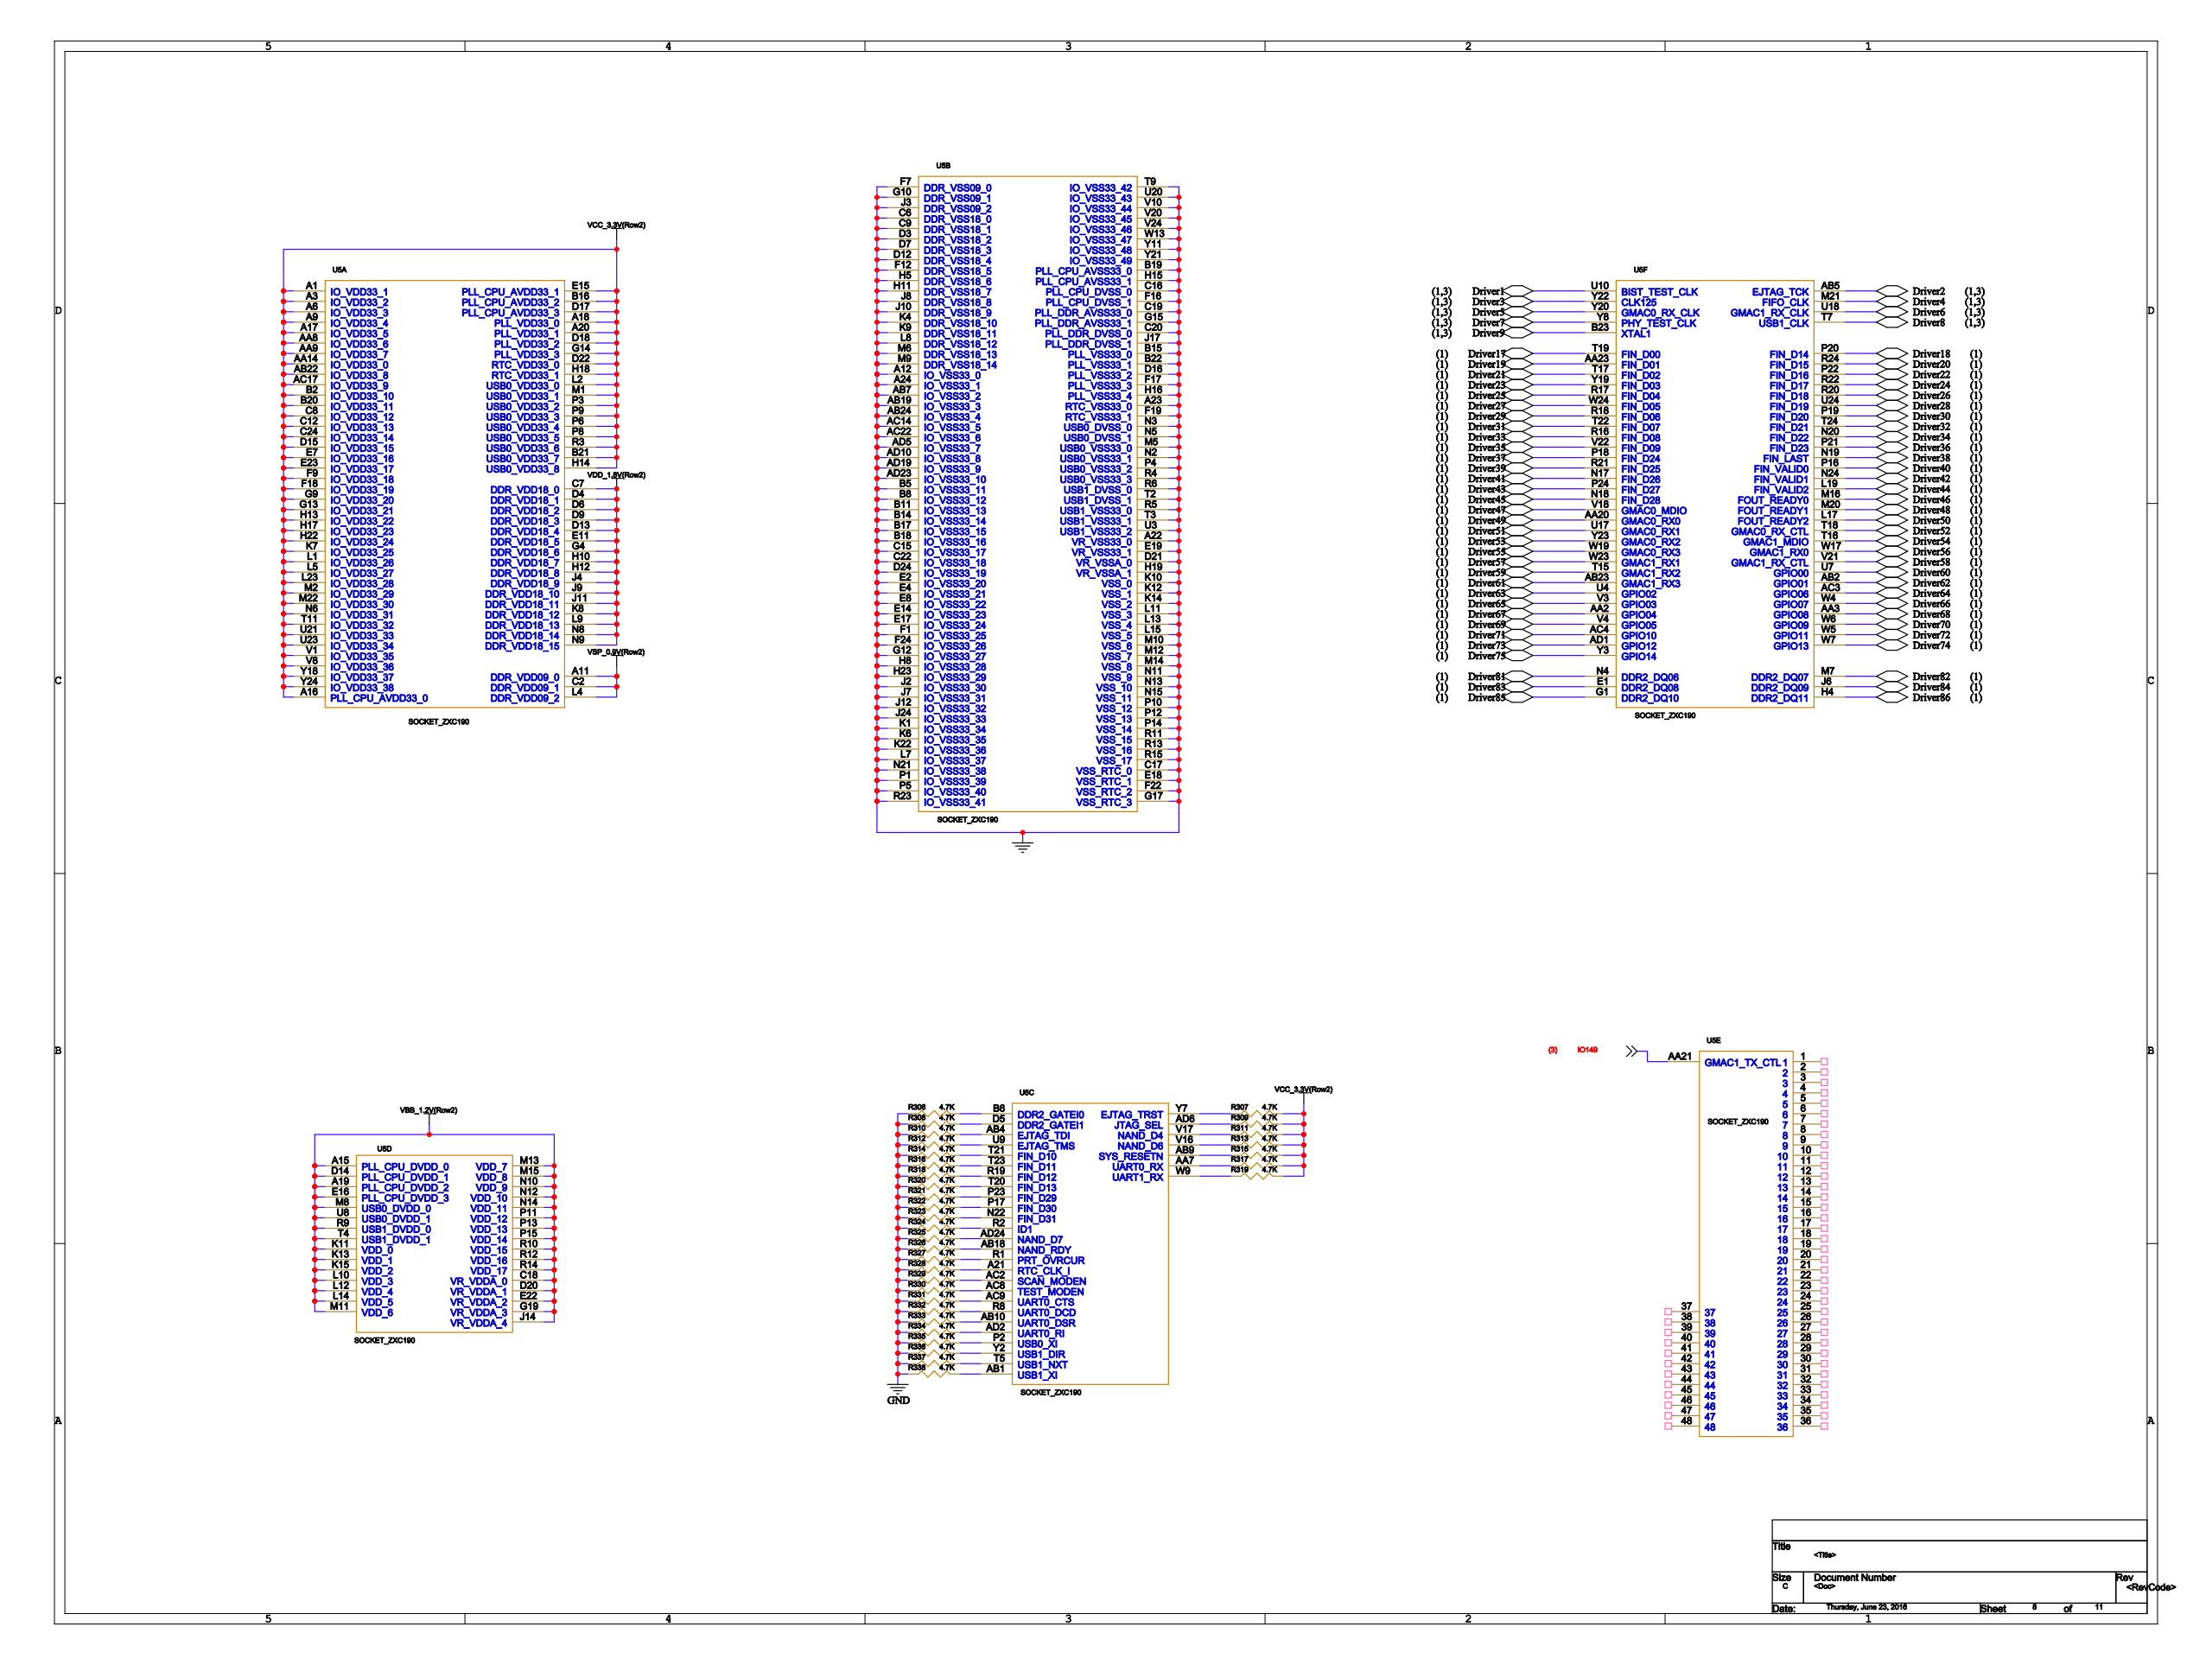Circuit board | Cadence Allegro | 531 parts | 624 nets | one sheet of the schematic
Parts on this sheet (reference | value | footprint):
R306 | 4.7K | R0805
R307 | 4.7K | R0805
R308 | 4.7K | R0805
R309 | 4.7K | R0805
R310 | 4.7K | R0805
R311 | 4.7K | R0805
R312 | 4.7K | R0805
R313 | 4.7K | R0805
R314 | 4.7K | R0805
R315 | 4.7K | R0805
R316 | 4.7K | R0805
R317 | 4.7K | R0805
R318 | 4.7K | R0805
R319 | 4.7K | R0805
R320 | 4.7K | R0805
R321 | 4.7K | R0805
R322 | 4.7K | R0805
R323 | 4.7K | R0805
R324 | 4.7K | R0805
R325 | 4.7K | R0805
R326 | 4.7K | R0805
R327 | 4.7K | R0805
R328 | 4.7K | R0805
R329 | 4.7K | R0805
R330 | 4.7K | R0805
R331 | 4.7K | R0805
R332 | 4.7K | R0805
R333 | 4.7K | R0805
R334 | 4.7K | R0805
R335 | 4.7K | R0805
R336 | 4.7K | R0805
R337 | 4.7K | R0805
R338 | 4.7K | R0805
U3 | SOCKET_ZXC190 | BGA-576
U4 | SOCKET_ZXC190 | BGA-576
U5 | SOCKET_ZXC190 | BGA-576
U10 | SOCKET_ZXC190 | BGA-576
Nets of these parts (net: part-pin ...):
GND: R306-1 R308-1 R310-1 R312-1 R314-1 R316-1 R318-1 R320-1 R321-1 R322-1 R323-1 R324-1 R325-1 R326-1 R327-1 R328-1 R329-1 R330-1 R331-1 R332-1 R333-1 R334-1 R335-1 R336-1 R337-1 R338-1 U3-A12 U3-A22 U3-A23 U3-A24 U3-AB7 U3-AB19 U3-AB24 U3-AC14 U3-AC22 U3-AD5 U3-AD10 U3-AD19 U3-AD23 U3-B5 U3-B8 U3-B11 U3-B14 U3-B15 U3-B17 U3-B18 U3-B19 U3-B22 U3-C6 U3-C9 U3-C15 U3-C16 U3-C17 U3-C19 U3-C20 U3-C22 U3-D3 U3-D7 U3-D12 U3-D16 U3-D21 U3-D24 U3-E2 U3-E4 U3-E8 U3-E14 U3-E17 U3-E18 U3-E19 U3-F1 U3-F7 U3-F12 U3-F16 U3-F17 U3-F19 U3-F22 U3-F24 U3-G10 U3-G12 U3-G15 U3-G17 U3-H5 U3-H8 U3-H11 U3-H15 U3-H16 U3-H19 U3-H23 U3-J2 U3-J3 U3-J7 U3-J8 U3-J10 U3-J12 U3-J17 U3-J24 U3-K1 U3-K4 U3-K6 U3-K9 U3-K10 U3-K12 U3-K14 U3-K22 U3-L7 U3-L8 U3-L11 U3-L13 U3-L15 U3-M5 U3-M6 U3-M9 U3-M10 U3-M12 U3-M14 U3-N2 U3-N3 U3-N5 U3-N11 U3-N13 U3-N15 U3-N21 U3-P1 U3-P4 U3-P5 U3-P10 U3-P12 U3-P14 U3-R4 U3-R5 U3-R6 U3-R11 U3-R13 U3-R15 U3-R23 U3-T2 U3-T3 U3-T9 U3-U3 U3-U20 U3-V10 U3-V20 U3-V24 U3-W13 U3-Y11 U3-Y21 U4-A12 U4-A22 U4-A23 U4-A24 U4-AB7 U4-AB19 U4-AB24 U4-AC14 U4-AC22 U4-AD5 U4-AD10 U4-AD19 U4-AD23 U4-B5 U4-B8 U4-B11 U4-B14 U4-B15 U4-B17 U4-B18 U4-B19 U4-B22 U4-C6 U4-C9 U4-C15 U4-C16 U4-C17 U4-C19 U4-C20 U4-C22 U4-D3 U4-D7 U4-D12 U4-D16 U4-D21 U4-D24 U4-E2 U4-E4 U4-E8 U4-E14 U4-E17 U4-E18 U4-E19 U4-F1 U4-F7 U4-F12 U4-F16 U4-F17 U4-F19 U4-F22 U4-F24 U4-G10 U4-G12 U4-G15 U4-G17 U4-H5 U4-H8 U4-H11 U4-H15 U4-H16 U4-H19 U4-H23 U4-J2 U4-J3 U4-J7 U4-J8 U4-J10 U4-J12 U4-J17 U4-J24 U4-K1 U4-K4 U4-K6 U4-K9 U4-K10 U4-K12 U4-K14 U4-K22 U4-L7 U4-L8 U4-L11 U4-L13 U4-L15 U4-M5 U4-M6 U4-M9 U4-M10 U4-M12 U4-M14 U4-N2 U4-N3 U4-N5 U4-N11 U4-N13 U4-N15 U4-N21 U4-P1 U4-P4 U4-P5 U4-P10 U4-P12 U4-P14 U4-R4 U4-R5 U4-R6 U4-R11 U4-R13 U4-R15 U4-R23 U4-T2 U4-T3 U4-T9 U4-U3 U4-U20 U4-V10 U4-V20 U4-V24 U4-W13 U4-Y11 U4-Y21 U5-A12 U5-A22 U5-A23 U5-A24 U5-AB7 U5-AB19 U5-AB24 U5-AC14 U5-AC22 U5-AD5 U5-AD10 U5-AD19 U5-AD23 U5-B5 U5-B8 U5-B11 U5-B14 U5-B15 U5-B17 U5-B18 U5-B19 U5-B22 U5-C6 U5-C9 U5-C15 U5-C16 U5-C17 U5-C19 U5-C20 U5-C22 U5-D3 U5-D7 U5-D12 U5-D16 U5-D21 U5-D24 U5-E2 U5-E4 U5-E8 U5-E14 U5-E17 U5-E18 U5-E19 U5-F1 U5-F7 U5-F12 U5-F16 U5-F17 U5-F19 U5-F22 U5-F24 U5-G10 U5-G12 U5-G15 U5-G17 U5-H5 U5-H8 U5-H11 U5-H15 U5-H16 U5-H19 U5-H23 U5-J2 U5-J3 U5-J7 U5-J8 U5-J10 U5-J12 U5-J17 U5-J24 U5-K1 U5-K4 U5-K6 U5-K9 U5-K10 U5-K12 U5-K14 U5-K22 U5-L7 U5-L8 U5-L11 U5-L13 U5-L15 U5-M5 U5-M6 U5-M9 U5-M10 U5-M12 U5-M14 U5-N2 U5-N3 U5-N5 U5-N11 U5-N13 U5-N15 U5-N21 U5-P1 U5-P4 U5-P5 U5-P10 U5-P12 U5-P14 U5-R4 U5-R5 U5-R6 U5-R11 U5-R13 U5-R15 U5-R23 U5-T2 U5-T3 U5-T9 U5-U3 U5-U20 U5-V10 U5-V20 U5-V24 U5-W13 U5-Y11 U5-Y21 U10-A12 U10-A22 U10-A23 U10-A24 U10-AB7 U10-AB19 U10-AB24 U10-AC14 U10-AC22 U10-AD5 U10-AD10 U10-AD19 U10-AD23 U10-B5 U10-B8 U10-B11 U10-B14 U10-B15 U10-B17 U10-B18 U10-B19 U10-B22 U10-C6 U10-C9 U10-C15 U10-C16 U10-C17 U10-C19 U10-C20 U10-C22 U10-D3 U10-D7 U10-D12 U10-D16 U10-D21 U10-D24 U10-E2 U10-E4 U10-E8 U10-E14 U10-E17 U10-E18 U10-E19 U10-F1 U10-F7 U10-F12 U10-F16 U10-F17 U10-F19 U10-F22 U10-F24 U10-G10 U10-G12 U10-G15 U10-G17 U10-H5 U10-H8 U10-H11 U10-H15 U10-H16 U10-H19 U10-H23 U10-J2 U10-J3 U10-J7 U10-J8 U10-J10 U10-J12 U10-J17 U10-J24 U10-K1 U10-K4 U10-K6 U10-K9 U10-K10 U10-K12 U10-K14 U10-K22 U10-L7 U10-L8 U10-L11 U10-L13 U10-L15 U10-M5 U10-M6 U10-M9 U10-M10 U10-M12 U10-M14 U10-N2 U10-N3 U10-N5 U10-N11 U10-N13 U10-N15 U10-N21 U10-P1 U10-P4 U10-P5 U10-P10 U10-P12 U10-P14 U10-R4 U10-R5 U10-R6 U10-R11 U10-R13 U10-R15 U10-R23 U10-T2 U10-T3 U10-T9 U10-U3 U10-U20 U10-V10 U10-V20 U10-V24 U10-W13 U10-Y11 U10-Y21
N8552845: R306-2 U5-B6
N8553269: R307-1 U5-Y7
VCC_3.3V(ROW2): R307-2 R309-2 R311-2 R313-2 R315-2 R317-2 R319-2 U5-A1 U5-A3 U5-A6 U5-A9 U5-A16 U5-A17 U5-A18 U5-A20 U5-AA8 U5-AA9 U5-AA14 U5-AB22 U5-AC17 U5-B2 U5-B16 U5-B20 U5-B21 U5-C8 U5-C12 U5-C24 U5-D15 U5-D17 U5-D18 U5-D22 U5-E7 U5-E15 U5-E23 U5-F9 U5-F18 U5-G9 U5-G13 U5-G14 U5-H13 U5-H14 U5-H17 U5-H18 U5-H22 U5-K7 U5-L1 U5-L2 U5-L5 U5-L23 U5-M1 U5-M2 U5-M22 U5-N6 U5-P3 U5-P6 U5-P8 U5-P9 U5-R3 U5-T11 U5-U21 U5-U23 U5-V1 U5-V8 U5-Y18 U5-Y24 U10-A1 U10-A3 U10-A6 U10-A9 U10-A16 U10-A17 U10-A18 U10-A20 U10-AA8 U10-AA9 U10-AA14 U10-AB22 U10-AC17 U10-B2 U10-B16 U10-B20 U10-B21 U10-C8 U10-C12 U10-C24 U10-D15 U10-D17 U10-D18 U10-D22 U10-E7 U10-E15 U10-E23 U10-F9 U10-F18 U10-G9 U10-G13 U10-G14 U10-H13 U10-H14 U10-H17 U10-H18 U10-H22 U10-K7 U10-L1 U10-L2 U10-L5 U10-L23 U10-M1 U10-M2 U10-M22 U10-N6 U10-P3 U10-P6 U10-P8 U10-P9 U10-R3 U10-T11 U10-U21 U10-U23 U10-V1 U10-V8 U10-Y18 U10-Y24
N8552841: R308-2 U5-D5
N8553305: R309-1 U5-AD6
N8552837: R310-2 U5-AB4
N8553449: R311-1 U5-V17
N8552833: R312-2 U5-U9
N8553453: R313-1 U5-V16
N8552829: R314-2 U5-T21
N8553477: R315-1 U5-AB9
N8552825: R316-2 U5-T23
N8553457: R317-1 U5-AA7
N8552821: R318-2 U5-R19
N8552801: R319-1 U5-W9
N8552877: R320-2 U5-T20
N8552873: R321-2 U5-P23
N8552869: R322-2 U5-P17
N8552865: R323-2 U5-N22
N8552861: R324-2 U5-R2
N8552857: R325-2 U5-AD24
N8552853: R326-2 U5-AB18
N8552849: R327-2 U5-R1
N8552905: R328-2 U5-A21
N8552901: R329-2 U5-AC2
N8552897: R330-2 U5-AC8
N8552893: R331-2 U5-AC9
N8553341: R332-2 U5-R8
N8552889: R333-2 U5-AB10
N8552885: R334-2 U5-AD2
N8552881: R335-2 U5-P2
N8552917: R336-2 U5-Y2
N8552913: R337-2 U5-T5
N8552909: R338-2 U5-AB1
IO149: U5-AA21